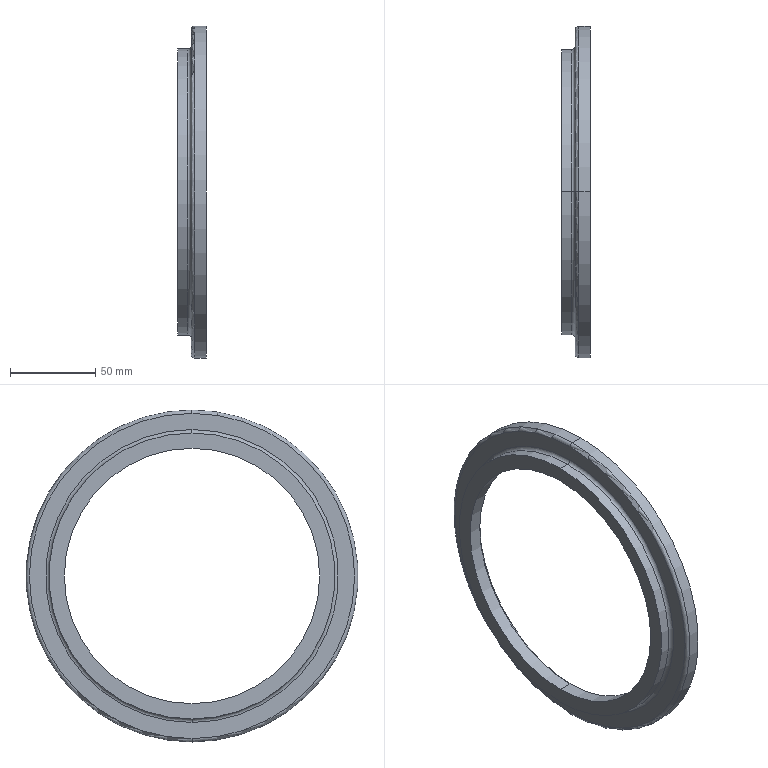Part | NX | features BREP 1 | 1 solid | 20 faces | box 17 x 195 x 195 mm | volume 90741 mm3 | cylinder 8 | torus 6 | plane 4 | cone 2 | commonest cylinder face diameters 150 x2 168 x2 180 x2 195 x2
STEP:
#1=CARTESIAN_POINT('',(6.,0.,84.));
#2=VERTEX_POINT('',#1);
#3=CARTESIAN_POINT('',(6.,0.,-84.));
#4=VERTEX_POINT('',#3);
#5=CARTESIAN_POINT('',(6.,0.,0.));
#6=DIRECTION('',(-1.,0.,0.));
#7=DIRECTION('',(0.,0.,1.));
#8=AXIS2_PLACEMENT_3D('',#5,#6,#7);
#9=CIRCLE('',#8,84.);
#10=EDGE_CURVE('',#2,#4,#9,.T.);
#11=ORIENTED_EDGE('',*,*,#10,.T.);
#12=CARTESIAN_POINT('',(0.,0.,-84.));
#13=VERTEX_POINT('',#12);
#14=CARTESIAN_POINT('',(0.,0.,-84.));
#15=DIRECTION('',(-1.,0.,0.));
#16=VECTOR('',#15,1000.);
#17=LINE('',#14,#16);
#18=EDGE_CURVE('',#4,#13,#17,.T.);
#19=ORIENTED_EDGE('',*,*,#18,.T.);
#20=CARTESIAN_POINT('',(0.,0.,84.));
#21=VERTEX_POINT('',#20);
#22=CARTESIAN_POINT('',(0.,0.,0.));
#23=DIRECTION('',(-1.,0.,0.));
#24=DIRECTION('',(0.,0.,1.));
#25=AXIS2_PLACEMENT_3D('',#22,#23,#24);
#26=CIRCLE('',#25,84.);
#27=EDGE_CURVE('',#21,#13,#26,.T.);
#28=ORIENTED_EDGE('',*,*,#27,.F.);
#29=CARTESIAN_POINT('',(0.,0.,84.));
#30=DIRECTION('',(-1.,0.,0.));
#31=VECTOR('',#30,1000.);
#32=LINE('',#29,#31);
#33=EDGE_CURVE('',#2,#21,#32,.T.);
#34=ORIENTED_EDGE('',*,*,#33,.F.);
#35=EDGE_LOOP('',(#11,#19,#28,#34));
#36=FACE_BOUND('',#35,.T.);
#37=CARTESIAN_POINT('',(0.,0.,0.));
#38=DIRECTION('',(-1.,0.,0.));
#39=DIRECTION('',(0.,0.,-1.));
#40=AXIS2_PLACEMENT_3D('',#37,#38,#39);
#41=CYLINDRICAL_SURFACE('',#40,84.);
#42=ADVANCED_FACE('',(#36),#41,.T.);
#43=CARTESIAN_POINT('',(6.,0.,0.));
#44=DIRECTION('',(-1.,0.,0.));
#45=DIRECTION('',(0.,0.,1.));
#46=AXIS2_PLACEMENT_3D('',#43,#44,#45);
#47=CIRCLE('',#46,84.);
#48=EDGE_CURVE('',#4,#2,#47,.T.);
#49=ORIENTED_EDGE('',*,*,#48,.F.);
#50=CARTESIAN_POINT('',(8.,0.,-86.));
#51=VERTEX_POINT('',#50);
#52=CARTESIAN_POINT('',(6.,0.,-86.));
#53=DIRECTION('',(0.,1.,0.));
#54=DIRECTION('',(0.,0.,1.));
#55=AXIS2_PLACEMENT_3D('',#52,#53,#54);
#56=CIRCLE('',#55,2.);
#57=EDGE_CURVE('',#4,#51,#56,.T.);
#58=ORIENTED_EDGE('',*,*,#57,.T.);
#59=CARTESIAN_POINT('',(8.,0.,86.));
#60=VERTEX_POINT('',#59);
#61=CARTESIAN_POINT('',(8.,0.,0.));
#62=DIRECTION('',(-1.,0.,0.));
#63=DIRECTION('',(0.,0.,1.));
#64=AXIS2_PLACEMENT_3D('',#61,#62,#63);
#65=CIRCLE('',#64,86.);
#66=EDGE_CURVE('',#51,#60,#65,.T.);
#67=ORIENTED_EDGE('',*,*,#66,.T.);
#68=CARTESIAN_POINT('',(6.,0.,86.));
#69=DIRECTION('',(0.,-1.,0.));
#70=DIRECTION('',(0.,0.,-1.));
#71=AXIS2_PLACEMENT_3D('',#68,#69,#70);
#72=CIRCLE('',#71,2.);
#73=EDGE_CURVE('',#2,#60,#72,.T.);
#74=ORIENTED_EDGE('',*,*,#73,.F.);
#75=EDGE_LOOP('',(#49,#58,#67,#74));
#76=FACE_BOUND('',#75,.T.);
#77=CARTESIAN_POINT('',(6.,0.,0.));
#78=DIRECTION('',(-1.,0.,0.));
#79=DIRECTION('',(0.,0.,-1.));
#80=AXIS2_PLACEMENT_3D('',#77,#78,#79);
#81=TOROIDAL_SURFACE('',#80,86.,2.);
#82=ADVANCED_FACE('',(#76),#81,.F.);
#83=CARTESIAN_POINT('',(10.,0.,97.5));
#84=VERTEX_POINT('',#83);
#85=CARTESIAN_POINT('',(10.,0.,-97.5));
#86=VERTEX_POINT('',#85);
#87=CARTESIAN_POINT('',(10.,0.,0.));
#88=DIRECTION('',(-1.,0.,0.));
#89=DIRECTION('',(0.,0.,1.));
#90=AXIS2_PLACEMENT_3D('',#87,#88,#89);
#91=CIRCLE('',#90,97.5);
#92=EDGE_CURVE('',#84,#86,#91,.T.);
#93=ORIENTED_EDGE('',*,*,#92,.T.);
#94=CARTESIAN_POINT('',(8.,0.,-95.5));
#95=VERTEX_POINT('',#94);
#96=CARTESIAN_POINT('',(10.,0.,-95.5));
#97=DIRECTION('',(0.,1.,0.));
#98=DIRECTION('',(0.,0.,1.));
#99=AXIS2_PLACEMENT_3D('',#96,#97,#98);
#100=CIRCLE('',#99,2.);
#101=EDGE_CURVE('',#86,#95,#100,.T.);
#102=ORIENTED_EDGE('',*,*,#101,.T.);
#103=CARTESIAN_POINT('',(8.,0.,95.5));
#104=VERTEX_POINT('',#103);
#105=CARTESIAN_POINT('',(8.,0.,0.));
#106=DIRECTION('',(-1.,0.,0.));
#107=DIRECTION('',(0.,0.,1.));
#108=AXIS2_PLACEMENT_3D('',#105,#106,#107);
#109=CIRCLE('',#108,95.5);
#110=EDGE_CURVE('',#104,#95,#109,.T.);
#111=ORIENTED_EDGE('',*,*,#110,.F.);
#112=CARTESIAN_POINT('',(10.,0.,95.5));
#113=DIRECTION('',(0.,-1.,0.));
#114=DIRECTION('',(0.,0.,-1.));
#115=AXIS2_PLACEMENT_3D('',#112,#113,#114);
#116=CIRCLE('',#115,2.);
#117=EDGE_CURVE('',#84,#104,#116,.T.);
#118=ORIENTED_EDGE('',*,*,#117,.F.);
#119=EDGE_LOOP('',(#93,#102,#111,#118));
#120=FACE_BOUND('',#119,.T.);
#121=CARTESIAN_POINT('',(10.,0.,0.));
#122=DIRECTION('',(-1.,0.,0.));
#123=DIRECTION('',(0.,0.,-1.));
#124=AXIS2_PLACEMENT_3D('',#121,#122,#123);
#125=TOROIDAL_SURFACE('',#124,95.5,2.);
#126=ADVANCED_FACE('',(#120),#125,.T.);
#127=CARTESIAN_POINT('',(17.,0.,97.5));
#128=VERTEX_POINT('',#127);
#129=CARTESIAN_POINT('',(17.,0.,-97.5));
#130=VERTEX_POINT('',#129);
#131=CARTESIAN_POINT('',(17.,0.,0.));
#132=DIRECTION('',(-1.,0.,0.));
#133=DIRECTION('',(0.,0.,1.));
#134=AXIS2_PLACEMENT_3D('',#131,#132,#133);
#135=CIRCLE('',#134,97.5);
#136=EDGE_CURVE('',#128,#130,#135,.T.);
#137=ORIENTED_EDGE('',*,*,#136,.T.);
#138=CARTESIAN_POINT('',(0.,0.,-97.5));
#139=DIRECTION('',(-1.,0.,0.));
#140=VECTOR('',#139,1000.);
#141=LINE('',#138,#140);
#142=EDGE_CURVE('',#130,#86,#141,.T.);
#143=ORIENTED_EDGE('',*,*,#142,.T.);
#144=ORIENTED_EDGE('',*,*,#92,.F.);
#145=CARTESIAN_POINT('',(0.,0.,97.5));
#146=DIRECTION('',(-1.,0.,0.));
#147=VECTOR('',#146,1000.);
#148=LINE('',#145,#147);
#149=EDGE_CURVE('',#128,#84,#148,.T.);
#150=ORIENTED_EDGE('',*,*,#149,.F.);
#151=EDGE_LOOP('',(#137,#143,#144,#150));
#152=FACE_BOUND('',#151,.T.);
#153=CARTESIAN_POINT('',(0.,0.,0.));
#154=DIRECTION('',(-1.,0.,0.));
#155=DIRECTION('',(0.,0.,-1.));
#156=AXIS2_PLACEMENT_3D('',#153,#154,#155);
#157=CYLINDRICAL_SURFACE('',#156,97.5);
#158=ADVANCED_FACE('',(#152),#157,.T.);
#159=CARTESIAN_POINT('',(17.,0.,-90.));
#160=VERTEX_POINT('',#159);
#161=CARTESIAN_POINT('',(17.,0.,90.));
#162=VERTEX_POINT('',#161);
#163=CARTESIAN_POINT('',(17.,0.,0.));
#164=DIRECTION('',(-1.,0.,0.));
#165=DIRECTION('',(0.,0.,1.));
#166=AXIS2_PLACEMENT_3D('',#163,#164,#165);
#167=CIRCLE('',#166,90.);
#168=EDGE_CURVE('',#160,#162,#167,.T.);
#169=ORIENTED_EDGE('',*,*,#168,.F.);
#170=CARTESIAN_POINT('',(12.,0.,-90.));
#171=VERTEX_POINT('',#170);
#172=CARTESIAN_POINT('',(0.,0.,-90.));
#173=DIRECTION('',(-1.,0.,0.));
#174=VECTOR('',#173,1000.);
#175=LINE('',#172,#174);
#176=EDGE_CURVE('',#160,#171,#175,.T.);
#177=ORIENTED_EDGE('',*,*,#176,.T.);
#178=CARTESIAN_POINT('',(12.,0.,90.));
#179=VERTEX_POINT('',#178);
#180=CARTESIAN_POINT('',(12.,0.,0.));
#181=DIRECTION('',(-1.,0.,0.));
#182=DIRECTION('',(0.,0.,1.));
#183=AXIS2_PLACEMENT_3D('',#180,#181,#182);
#184=CIRCLE('',#183,90.);
#185=EDGE_CURVE('',#171,#179,#184,.T.);
#186=ORIENTED_EDGE('',*,*,#185,.T.);
#187=CARTESIAN_POINT('',(0.,0.,90.));
#188=DIRECTION('',(-1.,0.,0.));
#189=VECTOR('',#188,1000.);
#190=LINE('',#187,#189);
#191=EDGE_CURVE('',#162,#179,#190,.T.);
#192=ORIENTED_EDGE('',*,*,#191,.F.);
#193=EDGE_LOOP('',(#169,#177,#186,#192));
#194=FACE_BOUND('',#193,.T.);
#195=CARTESIAN_POINT('',(0.,0.,0.));
#196=DIRECTION('',(-1.,0.,0.));
#197=DIRECTION('',(0.,0.,-1.));
#198=AXIS2_PLACEMENT_3D('',#195,#196,#197);
#199=CYLINDRICAL_SURFACE('',#198,90.);
#200=ADVANCED_FACE('',(#194),#199,.F.);
#201=ORIENTED_EDGE('',*,*,#185,.F.);
#202=CARTESIAN_POINT('',(10.,0.,-88.));
#203=VERTEX_POINT('',#202);
#204=CARTESIAN_POINT('',(12.,0.,-88.));
#205=DIRECTION('',(0.,1.,0.));
#206=DIRECTION('',(0.,0.,1.));
#207=AXIS2_PLACEMENT_3D('',#204,#205,#206);
#208=CIRCLE('',#207,2.);
#209=EDGE_CURVE('',#171,#203,#208,.T.);
#210=ORIENTED_EDGE('',*,*,#209,.T.);
#211=CARTESIAN_POINT('',(10.,0.,88.));
#212=VERTEX_POINT('',#211);
#213=CARTESIAN_POINT('',(10.,0.,0.));
#214=DIRECTION('',(-1.,0.,0.));
#215=DIRECTION('',(0.,0.,1.));
#216=AXIS2_PLACEMENT_3D('',#213,#214,#215);
#217=CIRCLE('',#216,88.);
#218=EDGE_CURVE('',#203,#212,#217,.T.);
#219=ORIENTED_EDGE('',*,*,#218,.T.);
#220=CARTESIAN_POINT('',(12.,0.,88.));
#221=DIRECTION('',(0.,-1.,0.));
#222=DIRECTION('',(0.,0.,-1.));
#223=AXIS2_PLACEMENT_3D('',#220,#221,#222);
#224=CIRCLE('',#223,2.);
#225=EDGE_CURVE('',#179,#212,#224,.T.);
#226=ORIENTED_EDGE('',*,*,#225,.F.);
#227=EDGE_LOOP('',(#201,#210,#219,#226));
#228=FACE_BOUND('',#227,.T.);
#229=CARTESIAN_POINT('',(12.,0.,0.));
#230=DIRECTION('',(-1.,0.,0.));
#231=DIRECTION('',(0.,0.,-1.));
#232=AXIS2_PLACEMENT_3D('',#229,#230,#231);
#233=TOROIDAL_SURFACE('',#232,88.,2.);
#234=ADVANCED_FACE('',(#228),#233,.F.);
#235=CARTESIAN_POINT('',(8.,0.,-75.));
#236=VERTEX_POINT('',#235);
#237=CARTESIAN_POINT('',(8.,0.,75.));
#238=VERTEX_POINT('',#237);
#239=CARTESIAN_POINT('',(8.,0.,0.));
#240=DIRECTION('',(-1.,0.,0.));
#241=DIRECTION('',(0.,0.,1.));
#242=AXIS2_PLACEMENT_3D('',#239,#240,#241);
#243=CIRCLE('',#242,75.);
#244=EDGE_CURVE('',#236,#238,#243,.T.);
#245=ORIENTED_EDGE('',*,*,#244,.T.);
#246=CARTESIAN_POINT('',(10.,0.,77.));
#247=VERTEX_POINT('',#246);
#248=CARTESIAN_POINT('',(8.,0.,75.));
#249=DIRECTION('',(0.7071,0.,0.7071));
#250=VECTOR('',#249,1000.);
#251=LINE('',#248,#250);
#252=EDGE_CURVE('',#247,#238,#251,.F.);
#253=ORIENTED_EDGE('',*,*,#252,.F.);
#254=CARTESIAN_POINT('',(10.,0.,-77.));
#255=VERTEX_POINT('',#254);
#256=CARTESIAN_POINT('',(10.,0.,0.));
#257=DIRECTION('',(-1.,0.,0.));
#258=DIRECTION('',(0.,0.,1.));
#259=AXIS2_PLACEMENT_3D('',#256,#257,#258);
#260=CIRCLE('',#259,77.);
#261=EDGE_CURVE('',#255,#247,#260,.T.);
#262=ORIENTED_EDGE('',*,*,#261,.F.);
#263=CARTESIAN_POINT('',(8.,0.,-75.));
#264=DIRECTION('',(0.7071,0.,-0.7071));
#265=VECTOR('',#264,1000.);
#266=LINE('',#263,#265);
#267=EDGE_CURVE('',#255,#236,#266,.F.);
#268=ORIENTED_EDGE('',*,*,#267,.T.);
#269=EDGE_LOOP('',(#245,#253,#262,#268));
#270=FACE_BOUND('',#269,.T.);
#271=CARTESIAN_POINT('',(8.,0.,0.));
#272=DIRECTION('',(1.,0.,0.));
#273=DIRECTION('',(0.,0.,1.));
#274=AXIS2_PLACEMENT_3D('',#271,#272,#273);
#275=CONICAL_SURFACE('',#274,75.,0.7854);
#276=ADVANCED_FACE('',(#270),#275,.F.);
#277=ORIENTED_EDGE('',*,*,#244,.F.);
#278=CARTESIAN_POINT('',(0.,0.,-75.));
#279=VERTEX_POINT('',#278);
#280=CARTESIAN_POINT('',(0.,0.,-75.));
#281=DIRECTION('',(-1.,0.,0.));
#282=VECTOR('',#281,1000.);
#283=LINE('',#280,#282);
#284=EDGE_CURVE('',#236,#279,#283,.T.);
#285=ORIENTED_EDGE('',*,*,#284,.T.);
#286=CARTESIAN_POINT('',(0.,0.,75.));
#287=VERTEX_POINT('',#286);
#288=CARTESIAN_POINT('',(0.,0.,0.));
#289=DIRECTION('',(-1.,0.,0.));
#290=DIRECTION('',(0.,0.,1.));
#291=AXIS2_PLACEMENT_3D('',#288,#289,#290);
#292=CIRCLE('',#291,75.);
#293=EDGE_CURVE('',#279,#287,#292,.T.);
#294=ORIENTED_EDGE('',*,*,#293,.T.);
#295=CARTESIAN_POINT('',(0.,0.,75.));
#296=DIRECTION('',(-1.,0.,0.));
#297=VECTOR('',#296,1000.);
#298=LINE('',#295,#297);
#299=EDGE_CURVE('',#238,#287,#298,.T.);
#300=ORIENTED_EDGE('',*,*,#299,.F.);
#301=EDGE_LOOP('',(#277,#285,#294,#300));
#302=FACE_BOUND('',#301,.T.);
#303=CARTESIAN_POINT('',(0.,0.,0.));
#304=DIRECTION('',(-1.,0.,0.));
#305=DIRECTION('',(0.,0.,-1.));
#306=AXIS2_PLACEMENT_3D('',#303,#304,#305);
#307=CYLINDRICAL_SURFACE('',#306,75.);
#308=ADVANCED_FACE('',(#302),#307,.F.);
#309=ORIENTED_EDGE('',*,*,#284,.F.);
#310=CARTESIAN_POINT('',(8.,0.,0.));
#311=DIRECTION('',(-1.,0.,0.));
#312=DIRECTION('',(0.,0.,1.));
#313=AXIS2_PLACEMENT_3D('',#310,#311,#312);
#314=CIRCLE('',#313,75.);
#315=EDGE_CURVE('',#238,#236,#314,.T.);
#316=ORIENTED_EDGE('',*,*,#315,.F.);
#317=ORIENTED_EDGE('',*,*,#299,.T.);
#318=CARTESIAN_POINT('',(0.,0.,0.));
#319=DIRECTION('',(-1.,0.,0.));
#320=DIRECTION('',(0.,0.,1.));
#321=AXIS2_PLACEMENT_3D('',#318,#319,#320);
#322=CIRCLE('',#321,75.);
#323=EDGE_CURVE('',#287,#279,#322,.T.);
#324=ORIENTED_EDGE('',*,*,#323,.T.);
#325=EDGE_LOOP('',(#309,#316,#317,#324));
#326=FACE_BOUND('',#325,.T.);
#327=CARTESIAN_POINT('',(0.,0.,0.));
#328=DIRECTION('',(-1.,0.,0.));
#329=DIRECTION('',(0.,0.,-1.));
#330=AXIS2_PLACEMENT_3D('',#327,#328,#329);
#331=CYLINDRICAL_SURFACE('',#330,75.);
#332=ADVANCED_FACE('',(#326),#331,.F.);
#333=ORIENTED_EDGE('',*,*,#252,.T.);
#334=ORIENTED_EDGE('',*,*,#315,.T.);
#335=ORIENTED_EDGE('',*,*,#267,.F.);
#336=CARTESIAN_POINT('',(10.,0.,0.));
#337=DIRECTION('',(-1.,0.,0.));
#338=DIRECTION('',(0.,0.,1.));
#339=AXIS2_PLACEMENT_3D('',#336,#337,#338);
#340=CIRCLE('',#339,77.);
#341=EDGE_CURVE('',#247,#255,#340,.T.);
#342=ORIENTED_EDGE('',*,*,#341,.F.);
#343=EDGE_LOOP('',(#333,#334,#335,#342));
#344=FACE_BOUND('',#343,.T.);
#345=CARTESIAN_POINT('',(8.,0.,0.));
#346=DIRECTION('',(1.,0.,0.));
#347=DIRECTION('',(0.,0.,1.));
#348=AXIS2_PLACEMENT_3D('',#345,#346,#347);
#349=CONICAL_SURFACE('',#348,75.,0.7854);
#350=ADVANCED_FACE('',(#344),#349,.F.);
#351=CARTESIAN_POINT('',(10.,0.,0.));
#352=DIRECTION('',(-1.,0.,0.));
#353=DIRECTION('',(0.,0.,1.));
#354=AXIS2_PLACEMENT_3D('',#351,#352,#353);
#355=CIRCLE('',#354,88.);
#356=EDGE_CURVE('',#212,#203,#355,.T.);
#357=ORIENTED_EDGE('',*,*,#356,.F.);
#358=ORIENTED_EDGE('',*,*,#218,.F.);
#359=EDGE_LOOP('',(#357,#358));
#360=FACE_BOUND('',#359,.T.);
#361=ORIENTED_EDGE('',*,*,#261,.T.);
#362=ORIENTED_EDGE('',*,*,#341,.T.);
#363=EDGE_LOOP('',(#361,#362));
#364=FACE_BOUND('',#363,.T.);
#365=CARTESIAN_POINT('',(10.,88.,0.));
#366=DIRECTION('',(-1.,0.,0.));
#367=DIRECTION('',(0.,0.,-1.));
#368=AXIS2_PLACEMENT_3D('',#365,#366,#367);
#369=PLANE('',#368);
#370=ADVANCED_FACE('',(#360,#364),#369,.F.);
#371=ORIENTED_EDGE('',*,*,#209,.F.);
#372=CARTESIAN_POINT('',(12.,0.,0.));
#373=DIRECTION('',(-1.,0.,0.));
#374=DIRECTION('',(0.,0.,1.));
#375=AXIS2_PLACEMENT_3D('',#372,#373,#374);
#376=CIRCLE('',#375,90.);
#377=EDGE_CURVE('',#179,#171,#376,.T.);
#378=ORIENTED_EDGE('',*,*,#377,.F.);
#379=ORIENTED_EDGE('',*,*,#225,.T.);
#380=ORIENTED_EDGE('',*,*,#356,.T.);
#381=EDGE_LOOP('',(#371,#378,#379,#380));
#382=FACE_BOUND('',#381,.T.);
#383=CARTESIAN_POINT('',(12.,0.,0.));
#384=DIRECTION('',(-1.,0.,0.));
#385=DIRECTION('',(0.,0.,-1.));
#386=AXIS2_PLACEMENT_3D('',#383,#384,#385);
#387=TOROIDAL_SURFACE('',#386,88.,2.);
#388=ADVANCED_FACE('',(#382),#387,.F.);
#389=ORIENTED_EDGE('',*,*,#176,.F.);
#390=CARTESIAN_POINT('',(17.,0.,0.));
#391=DIRECTION('',(-1.,0.,0.));
#392=DIRECTION('',(0.,0.,1.));
#393=AXIS2_PLACEMENT_3D('',#390,#391,#392);
#394=CIRCLE('',#393,90.);
#395=EDGE_CURVE('',#162,#160,#394,.T.);
#396=ORIENTED_EDGE('',*,*,#395,.F.);
#397=ORIENTED_EDGE('',*,*,#191,.T.);
#398=ORIENTED_EDGE('',*,*,#377,.T.);
#399=EDGE_LOOP('',(#389,#396,#397,#398));
#400=FACE_BOUND('',#399,.T.);
#401=CARTESIAN_POINT('',(0.,0.,0.));
#402=DIRECTION('',(-1.,0.,0.));
#403=DIRECTION('',(0.,0.,-1.));
#404=AXIS2_PLACEMENT_3D('',#401,#402,#403);
#405=CYLINDRICAL_SURFACE('',#404,90.);
#406=ADVANCED_FACE('',(#400),#405,.F.);
#407=ORIENTED_EDGE('',*,*,#136,.F.);
#408=CARTESIAN_POINT('',(17.,0.,0.));
#409=DIRECTION('',(-1.,0.,0.));
#410=DIRECTION('',(0.,0.,1.));
#411=AXIS2_PLACEMENT_3D('',#408,#409,#410);
#412=CIRCLE('',#411,97.5);
#413=EDGE_CURVE('',#130,#128,#412,.T.);
#414=ORIENTED_EDGE('',*,*,#413,.F.);
#415=EDGE_LOOP('',(#407,#414));
#416=FACE_BOUND('',#415,.T.);
#417=ORIENTED_EDGE('',*,*,#395,.T.);
#418=ORIENTED_EDGE('',*,*,#168,.T.);
#419=EDGE_LOOP('',(#417,#418));
#420=FACE_BOUND('',#419,.T.);
#421=CARTESIAN_POINT('',(17.,97.5,0.));
#422=DIRECTION('',(-1.,0.,0.));
#423=DIRECTION('',(0.,0.,-1.));
#424=AXIS2_PLACEMENT_3D('',#421,#422,#423);
#425=PLANE('',#424);
#426=ADVANCED_FACE('',(#416,#420),#425,.F.);
#427=ORIENTED_EDGE('',*,*,#142,.F.);
#428=ORIENTED_EDGE('',*,*,#413,.T.);
#429=ORIENTED_EDGE('',*,*,#149,.T.);
#430=CARTESIAN_POINT('',(10.,0.,0.));
#431=DIRECTION('',(-1.,0.,0.));
#432=DIRECTION('',(0.,0.,1.));
#433=AXIS2_PLACEMENT_3D('',#430,#431,#432);
#434=CIRCLE('',#433,97.5);
#435=EDGE_CURVE('',#86,#84,#434,.T.);
#436=ORIENTED_EDGE('',*,*,#435,.F.);
#437=EDGE_LOOP('',(#427,#428,#429,#436));
#438=FACE_BOUND('',#437,.T.);
#439=CARTESIAN_POINT('',(0.,0.,0.));
#440=DIRECTION('',(-1.,0.,0.));
#441=DIRECTION('',(0.,0.,-1.));
#442=AXIS2_PLACEMENT_3D('',#439,#440,#441);
#443=CYLINDRICAL_SURFACE('',#442,97.5);
#444=ADVANCED_FACE('',(#438),#443,.T.);
#445=ORIENTED_EDGE('',*,*,#101,.F.);
#446=ORIENTED_EDGE('',*,*,#435,.T.);
#447=ORIENTED_EDGE('',*,*,#117,.T.);
#448=CARTESIAN_POINT('',(8.,0.,0.));
#449=DIRECTION('',(-1.,0.,0.));
#450=DIRECTION('',(0.,0.,1.));
#451=AXIS2_PLACEMENT_3D('',#448,#449,#450);
#452=CIRCLE('',#451,95.5);
#453=EDGE_CURVE('',#95,#104,#452,.T.);
#454=ORIENTED_EDGE('',*,*,#453,.F.);
#455=EDGE_LOOP('',(#445,#446,#447,#454));
#456=FACE_BOUND('',#455,.T.);
#457=CARTESIAN_POINT('',(10.,0.,0.));
#458=DIRECTION('',(-1.,0.,0.));
#459=DIRECTION('',(0.,0.,-1.));
#460=AXIS2_PLACEMENT_3D('',#457,#458,#459);
#461=TOROIDAL_SURFACE('',#460,95.5,2.);
#462=ADVANCED_FACE('',(#456),#461,.T.);
#463=CARTESIAN_POINT('',(8.,0.,0.));
#464=DIRECTION('',(-1.,0.,0.));
#465=DIRECTION('',(0.,0.,1.));
#466=AXIS2_PLACEMENT_3D('',#463,#464,#465);
#467=CIRCLE('',#466,86.);
#468=EDGE_CURVE('',#60,#51,#467,.T.);
#469=ORIENTED_EDGE('',*,*,#468,.F.);
#470=ORIENTED_EDGE('',*,*,#66,.F.);
#471=EDGE_LOOP('',(#469,#470));
#472=FACE_BOUND('',#471,.T.);
#473=ORIENTED_EDGE('',*,*,#110,.T.);
#474=ORIENTED_EDGE('',*,*,#453,.T.);
#475=EDGE_LOOP('',(#473,#474));
#476=FACE_BOUND('',#475,.T.);
#477=CARTESIAN_POINT('',(8.,86.,0.));
#478=DIRECTION('',(1.,0.,0.));
#479=DIRECTION('',(0.,0.,1.));
#480=AXIS2_PLACEMENT_3D('',#477,#478,#479);
#481=PLANE('',#480);
#482=ADVANCED_FACE('',(#472,#476),#481,.F.);
#483=ORIENTED_EDGE('',*,*,#57,.F.);
#484=ORIENTED_EDGE('',*,*,#10,.F.);
#485=ORIENTED_EDGE('',*,*,#73,.T.);
#486=ORIENTED_EDGE('',*,*,#468,.T.);
#487=EDGE_LOOP('',(#483,#484,#485,#486));
#488=FACE_BOUND('',#487,.T.);
#489=CARTESIAN_POINT('',(6.,0.,0.));
#490=DIRECTION('',(-1.,0.,0.));
#491=DIRECTION('',(0.,0.,-1.));
#492=AXIS2_PLACEMENT_3D('',#489,#490,#491);
#493=TOROIDAL_SURFACE('',#492,86.,2.);
#494=ADVANCED_FACE('',(#488),#493,.F.);
#495=ORIENTED_EDGE('',*,*,#18,.F.);
#496=ORIENTED_EDGE('',*,*,#48,.T.);
#497=ORIENTED_EDGE('',*,*,#33,.T.);
#498=CARTESIAN_POINT('',(0.,0.,0.));
#499=DIRECTION('',(-1.,0.,0.));
#500=DIRECTION('',(0.,0.,1.));
#501=AXIS2_PLACEMENT_3D('',#498,#499,#500);
#502=CIRCLE('',#501,84.);
#503=EDGE_CURVE('',#13,#21,#502,.T.);
#504=ORIENTED_EDGE('',*,*,#503,.F.);
#505=EDGE_LOOP('',(#495,#496,#497,#504));
#506=FACE_BOUND('',#505,.T.);
#507=CARTESIAN_POINT('',(0.,0.,0.));
#508=DIRECTION('',(-1.,0.,0.));
#509=DIRECTION('',(0.,0.,-1.));
#510=AXIS2_PLACEMENT_3D('',#507,#508,#509);
#511=CYLINDRICAL_SURFACE('',#510,84.);
#512=ADVANCED_FACE('',(#506),#511,.T.);
#513=ORIENTED_EDGE('',*,*,#323,.F.);
#514=ORIENTED_EDGE('',*,*,#293,.F.);
#515=EDGE_LOOP('',(#513,#514));
#516=FACE_BOUND('',#515,.T.);
#517=ORIENTED_EDGE('',*,*,#27,.T.);
#518=ORIENTED_EDGE('',*,*,#503,.T.);
#519=EDGE_LOOP('',(#517,#518));
#520=FACE_BOUND('',#519,.T.);
#521=CARTESIAN_POINT('',(0.,75.,0.));
#522=DIRECTION('',(1.,0.,0.));
#523=DIRECTION('',(0.,0.,1.));
#524=AXIS2_PLACEMENT_3D('',#521,#522,#523);
#525=PLANE('',#524);
#526=ADVANCED_FACE('',(#516,#520),#525,.F.);
#527=CLOSED_SHELL('',(#42,#82,#126,#158,#200,#234,#276,#308,#332,#350,#370,#388,#406,#426,#444,#462,#482,#494,#512,#526));
#528=MANIFOLD_SOLID_BREP('',#527);
#529=(LENGTH_UNIT()NAMED_UNIT(*)SI_UNIT(.MILLI.,.METRE.));
#530=UNCERTAINTY_MEASURE_WITH_UNIT(LENGTH_MEASURE(0.00001),#529,'','');
#531=(NAMED_UNIT(*)PLANE_ANGLE_UNIT()SI_UNIT($,.RADIAN.));
#532=(NAMED_UNIT(*)SI_UNIT($,.STERADIAN.)SOLID_ANGLE_UNIT());
#533=(GEOMETRIC_REPRESENTATION_CONTEXT(3)GLOBAL_UNCERTAINTY_ASSIGNED_CONTEXT((#530))GLOBAL_UNIT_ASSIGNED_CONTEXT((#529,#531,#532))REPRESENTATION_CONTEXT('',''));
#534=ADVANCED_BREP_SHAPE_REPRESENTATION('',(#528),#533);